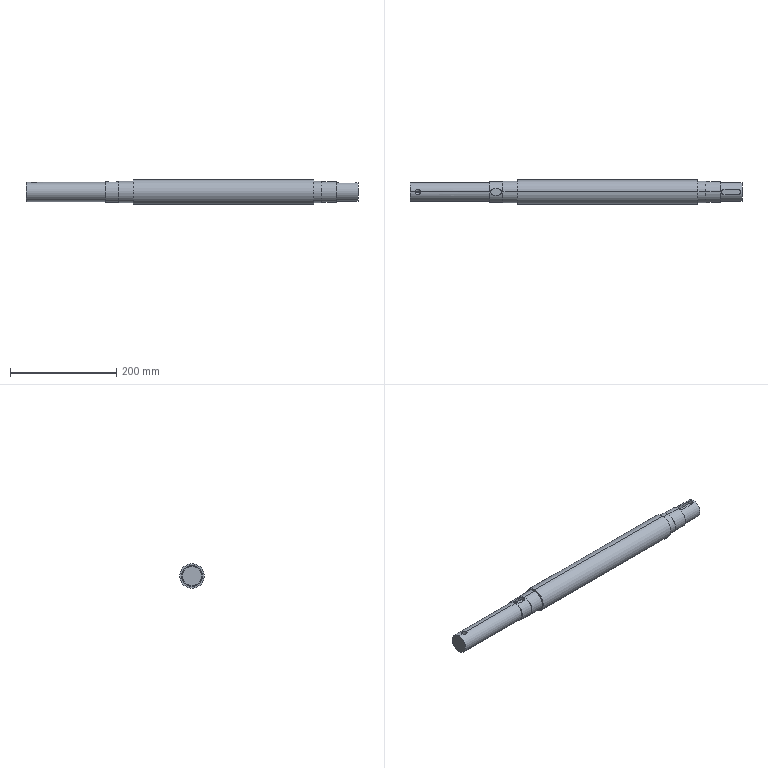Part | SolidWorks | features ICE 8, HoleWzd 2, Extrusion 1 | 1 solid | 42 faces | box 625 x 46 x 46 mm | volume 866135 mm3 | cylinder 24 | plane 14 | cone 4 | commonest cylinder face diameters 39 x4 40 x4 10 x3 12 x3 8.5 x2 10.2 x2
STEP:
#1=CARTESIAN_POINT('',(-44.,6.,18.554));
#2=VERTEX_POINT('',#1);
#3=CARTESIAN_POINT('',(-50.,0.,19.5));
#4=VERTEX_POINT('',#3);
#5=CARTESIAN_POINT('',(-44.,6.,18.554));
#6=CARTESIAN_POINT('',(-44.399,6.,18.554));
#7=CARTESIAN_POINT('',(-44.791,5.961,18.567));
#8=CARTESIAN_POINT('',(-45.369,5.845,18.603));
#9=CARTESIAN_POINT('',(-45.56,5.797,18.618));
#10=CARTESIAN_POINT('',(-45.938,5.682,18.654));
#11=CARTESIAN_POINT('',(-46.125,5.614,18.674));
#12=CARTESIAN_POINT('',(-46.669,5.388,18.742));
#13=CARTESIAN_POINT('',(-47.013,5.203,18.794));
#14=CARTESIAN_POINT('',(-47.501,4.877,18.881));
#15=CARTESIAN_POINT('',(-47.66,4.759,18.911));
#16=CARTESIAN_POINT('',(-47.963,4.51,18.972));
#17=CARTESIAN_POINT('',(-48.107,4.378,19.003));
#18=CARTESIAN_POINT('',(-48.519,3.966,19.095));
#19=CARTESIAN_POINT('',(-48.767,3.665,19.155));
#20=CARTESIAN_POINT('',(-49.206,3.009,19.269));
#21=CARTESIAN_POINT('',(-49.39,2.664,19.321));
#22=CARTESIAN_POINT('',(-49.615,2.123,19.385));
#23=CARTESIAN_POINT('',(-49.682,1.938,19.404));
#24=CARTESIAN_POINT('',(-49.797,1.561,19.438));
#25=CARTESIAN_POINT('',(-49.845,1.367,19.453));
#26=CARTESIAN_POINT('',(-49.962,0.7854,19.488));
#27=CARTESIAN_POINT('',(-50.,0.3942,19.5));
#28=CARTESIAN_POINT('',(-50.,0.,19.5));
#29=B_SPLINE_CURVE_WITH_KNOTS('',3,(#5,#6,#7,#8,#9,#10,#11,#12,#13,#14,#15,#16,#17,#18,#19,#20,#21,#22,#23,#24,#25,#26,#27,#28),.UNSPECIFIED.,.F.,.F.,(4,2,2,2,2,2,2,2,2,2,2,4),(0.,0.00118,0.00177,0.00236,0.00354,0.00413,0.00472,0.0059,0.00708,0.00767,0.008259,0.009439),.UNSPECIFIED.);
#30=EDGE_CURVE('',#2,#4,#29,.T.);
#31=ORIENTED_EDGE('',*,*,#30,.T.);
#32=CARTESIAN_POINT('',(-50.,0.,13.55));
#33=VERTEX_POINT('',#32);
#34=CARTESIAN_POINT('',(-50.,0.,22.5));
#35=DIRECTION('',(0.,0.,-1.));
#36=VECTOR('',#35,1000.);
#37=LINE('',#34,#36);
#38=EDGE_CURVE('',#4,#33,#37,.T.);
#39=ORIENTED_EDGE('',*,*,#38,.T.);
#40=CARTESIAN_POINT('',(-44.,6.,13.55));
#41=VERTEX_POINT('',#40);
#42=CARTESIAN_POINT('',(-44.,0.,13.55));
#43=DIRECTION('',(0.,0.,1.));
#44=DIRECTION('',(1.,0.,0.));
#45=AXIS2_PLACEMENT_3D('',#42,#43,#44);
#46=CIRCLE('',#45,6.);
#47=EDGE_CURVE('',#41,#33,#46,.T.);
#48=ORIENTED_EDGE('',*,*,#47,.F.);
#49=CARTESIAN_POINT('',(-44.,6.,22.5));
#50=DIRECTION('',(0.,0.,-1.));
#51=VECTOR('',#50,1000.);
#52=LINE('',#49,#51);
#53=EDGE_CURVE('',#2,#41,#52,.T.);
#54=ORIENTED_EDGE('',*,*,#53,.F.);
#55=EDGE_LOOP('',(#31,#39,#48,#54));
#56=FACE_OUTER_BOUND('',#55,.T.);
#57=CARTESIAN_POINT('',(-44.,0.,22.5));
#58=DIRECTION('',(0.,0.,-1.));
#59=DIRECTION('',(-1.,0.,0.));
#60=AXIS2_PLACEMENT_3D('',#57,#58,#59);
#61=CYLINDRICAL_SURFACE('',#60,6.);
#62=ADVANCED_FACE('',(#56),#61,.F.);
#63=CARTESIAN_POINT('',(403.,0.,4.25));
#64=VERTEX_POINT('',#63);
#65=CARTESIAN_POINT('',(403.,0.,-4.25));
#66=VERTEX_POINT('',#65);
#67=CARTESIAN_POINT('',(403.,0.,0.));
#68=DIRECTION('',(1.,0.,0.));
#69=DIRECTION('',(0.,0.,-1.));
#70=AXIS2_PLACEMENT_3D('',#67,#68,#69);
#71=CIRCLE('',#70,4.25);
#72=EDGE_CURVE('',#64,#66,#71,.T.);
#73=ORIENTED_EDGE('',*,*,#72,.F.);
#74=CARTESIAN_POINT('',(423.,0.,4.25));
#75=VERTEX_POINT('',#74);
#76=CARTESIAN_POINT('',(423.,0.,4.25));
#77=DIRECTION('',(1.,0.,0.));
#78=VECTOR('',#77,1000.);
#79=LINE('',#76,#78);
#80=EDGE_CURVE('',#64,#75,#79,.T.);
#81=ORIENTED_EDGE('',*,*,#80,.T.);
#82=CARTESIAN_POINT('',(423.,0.,-4.25));
#83=VERTEX_POINT('',#82);
#84=CARTESIAN_POINT('',(423.,0.,0.));
#85=DIRECTION('',(1.,0.,0.));
#86=DIRECTION('',(0.,0.,-1.));
#87=AXIS2_PLACEMENT_3D('',#84,#85,#86);
#88=CIRCLE('',#87,4.25);
#89=EDGE_CURVE('',#75,#83,#88,.T.);
#90=ORIENTED_EDGE('',*,*,#89,.T.);
#91=CARTESIAN_POINT('',(423.,0.,-4.25));
#92=DIRECTION('',(1.,0.,0.));
#93=VECTOR('',#92,1000.);
#94=LINE('',#91,#93);
#95=EDGE_CURVE('',#66,#83,#94,.T.);
#96=ORIENTED_EDGE('',*,*,#95,.F.);
#97=EDGE_LOOP('',(#73,#81,#90,#96));
#98=FACE_OUTER_BOUND('',#97,.T.);
#99=CARTESIAN_POINT('',(423.,0.,0.));
#100=DIRECTION('',(1.,0.,0.));
#101=DIRECTION('',(0.,0.,-1.));
#102=AXIS2_PLACEMENT_3D('',#99,#100,#101);
#103=CYLINDRICAL_SURFACE('',#102,4.25);
#104=ADVANCED_FACE('',(#98),#103,.F.);
#105=CARTESIAN_POINT('',(400.446,0.,0.));
#106=VERTEX_POINT('',#105);
#107=CARTESIAN_POINT('',(403.,0.,-4.25));
#108=DIRECTION('',(0.515,0.,-0.8572));
#109=VECTOR('',#108,1000.);
#110=LINE('',#107,#109);
#111=EDGE_CURVE('',#106,#66,#110,.T.);
#112=ORIENTED_EDGE('',*,*,#111,.F.);
#113=CARTESIAN_POINT('',(403.,0.,4.25));
#114=DIRECTION('',(0.515,0.,0.8572));
#115=VECTOR('',#114,1000.);
#116=LINE('',#113,#115);
#117=EDGE_CURVE('',#106,#64,#116,.T.);
#118=ORIENTED_EDGE('',*,*,#117,.T.);
#119=ORIENTED_EDGE('',*,*,#72,.T.);
#120=EDGE_LOOP('',(#112,#118,#119));
#121=FACE_OUTER_BOUND('',#120,.T.);
#122=CARTESIAN_POINT('',(403.,0.,0.));
#123=DIRECTION('',(1.,0.,0.));
#124=DIRECTION('',(0.,0.,-1.));
#125=AXIS2_PLACEMENT_3D('',#122,#123,#124);
#126=CONICAL_SURFACE('',#125,4.25,1.03);
#127=ADVANCED_FACE('',(#121),#126,.F.);
#128=CARTESIAN_POINT('',(-187.,0.,-5.064));
#129=VERTEX_POINT('',#128);
#130=CARTESIAN_POINT('',(-181.9,0.,-2.));
#131=VERTEX_POINT('',#130);
#132=CARTESIAN_POINT('',(-181.9,0.,-2.));
#133=DIRECTION('',(0.8572,0.,0.515));
#134=VECTOR('',#133,1000.);
#135=LINE('',#132,#134);
#136=EDGE_CURVE('',#129,#131,#135,.T.);
#137=ORIENTED_EDGE('',*,*,#136,.F.);
#138=CARTESIAN_POINT('',(-192.1,0.,-2.));
#139=VERTEX_POINT('',#138);
#140=CARTESIAN_POINT('',(-192.1,0.,-2.));
#141=DIRECTION('',(-0.8572,0.,0.515));
#142=VECTOR('',#141,1000.);
#143=LINE('',#140,#142);
#144=EDGE_CURVE('',#129,#139,#143,.T.);
#145=ORIENTED_EDGE('',*,*,#144,.T.);
#146=CARTESIAN_POINT('',(-187.,0.,-2.));
#147=DIRECTION('',(0.,0.,1.));
#148=DIRECTION('',(1.,0.,0.));
#149=AXIS2_PLACEMENT_3D('',#146,#147,#148);
#150=CIRCLE('',#149,5.1);
#151=EDGE_CURVE('',#139,#131,#150,.T.);
#152=ORIENTED_EDGE('',*,*,#151,.T.);
#153=EDGE_LOOP('',(#137,#145,#152));
#154=FACE_OUTER_BOUND('',#153,.T.);
#155=CARTESIAN_POINT('',(-187.,0.,-2.));
#156=DIRECTION('',(0.,0.,1.));
#157=DIRECTION('',(1.,0.,0.));
#158=AXIS2_PLACEMENT_3D('',#155,#156,#157);
#159=CONICAL_SURFACE('',#158,5.1,1.03);
#160=ADVANCED_FACE('',(#154),#159,.F.);
#161=ORIENTED_EDGE('',*,*,#151,.F.);
#162=CARTESIAN_POINT('',(-192.1,0.,18.));
#163=VERTEX_POINT('',#162);
#164=CARTESIAN_POINT('',(-192.1,0.,18.));
#165=DIRECTION('',(0.,0.,1.));
#166=VECTOR('',#165,1000.);
#167=LINE('',#164,#166);
#168=EDGE_CURVE('',#139,#163,#167,.T.);
#169=ORIENTED_EDGE('',*,*,#168,.T.);
#170=CARTESIAN_POINT('',(-181.9,0.,18.));
#171=VERTEX_POINT('',#170);
#172=CARTESIAN_POINT('',(-181.9,0.,18.));
#173=CARTESIAN_POINT('',(-181.9,-0.3388,18.));
#174=CARTESIAN_POINT('',(-181.933,-0.6717,17.99));
#175=CARTESIAN_POINT('',(-182.064,-1.326,17.954));
#176=CARTESIAN_POINT('',(-182.163,-1.651,17.927));
#177=CARTESIAN_POINT('',(-182.42,-2.268,17.859));
#178=CARTESIAN_POINT('',(-182.577,-2.56,17.819));
#179=CARTESIAN_POINT('',(-182.947,-3.113,17.731));
#180=CARTESIAN_POINT('',(-183.161,-3.374,17.683));
#181=CARTESIAN_POINT('',(-183.629,-3.841,17.587));
#182=CARTESIAN_POINT('',(-183.885,-4.052,17.539));
#183=CARTESIAN_POINT('',(-184.442,-4.425,17.449));
#184=CARTESIAN_POINT('',(-184.736,-4.582,17.408));
#185=CARTESIAN_POINT('',(-185.195,-4.773,17.356));
#186=CARTESIAN_POINT('',(-185.352,-4.829,17.34));
#187=CARTESIAN_POINT('',(-185.672,-4.927,17.313));
#188=CARTESIAN_POINT('',(-185.837,-4.968,17.301));
#189=CARTESIAN_POINT('',(-186.331,-5.067,17.272));
#190=CARTESIAN_POINT('',(-186.663,-5.1,17.262));
#191=CARTESIAN_POINT('',(-187.332,-5.1,17.262));
#192=CARTESIAN_POINT('',(-187.672,-5.067,17.272));
#193=CARTESIAN_POINT('',(-188.328,-4.935,17.31));
#194=CARTESIAN_POINT('',(-188.647,-4.839,17.338));
#195=CARTESIAN_POINT('',(-189.266,-4.581,17.408));
#196=CARTESIAN_POINT('',(-189.562,-4.422,17.449));
#197=CARTESIAN_POINT('',(-190.112,-4.054,17.539));
#198=CARTESIAN_POINT('',(-190.372,-3.841,17.587));
#199=CARTESIAN_POINT('',(-190.843,-3.369,17.683));
#200=CARTESIAN_POINT('',(-191.053,-3.114,17.731));
#201=CARTESIAN_POINT('',(-191.422,-2.563,17.819));
#202=CARTESIAN_POINT('',(-191.582,-2.264,17.86));
#203=CARTESIAN_POINT('',(-191.838,-1.649,17.927));
#204=CARTESIAN_POINT('',(-191.935,-1.331,17.954));
#205=CARTESIAN_POINT('',(-192.034,-0.837,17.981));
#206=CARTESIAN_POINT('',(-192.059,-0.6688,17.988));
#207=CARTESIAN_POINT('',(-192.092,-0.3341,17.998));
#208=CARTESIAN_POINT('',(-192.1,-0.167,18.));
#209=CARTESIAN_POINT('',(-192.1,0.,18.));
#210=B_SPLINE_CURVE_WITH_KNOTS('',3,(#172,#173,#174,#175,#176,#177,#178,#179,#180,#181,#182,#183,#184,#185,#186,#187,#188,#189,#190,#191,#192,#193,#194,#195,#196,#197,#198,#199,#200,#201,#202,#203,#204,#205,#206,#207,#208,#209),.UNSPECIFIED.,.F.,.F.,(4,2,2,2,2,2,2,2,2,2,2,2,2,2,2,2,2,2,4),(0.,0.001002,0.002003,0.003005,0.004007,0.005009,0.00601,0.006511,0.007012,0.008014,0.009015,0.01002,0.01102,0.01202,0.01302,0.01402,0.01503,0.01553,0.01603),.UNSPECIFIED.);
#211=EDGE_CURVE('',#171,#163,#210,.T.);
#212=ORIENTED_EDGE('',*,*,#211,.F.);
#213=CARTESIAN_POINT('',(-181.9,0.,18.));
#214=DIRECTION('',(0.,0.,1.));
#215=VECTOR('',#214,1000.);
#216=LINE('',#213,#215);
#217=EDGE_CURVE('',#131,#171,#216,.T.);
#218=ORIENTED_EDGE('',*,*,#217,.F.);
#219=EDGE_LOOP('',(#161,#169,#212,#218));
#220=FACE_OUTER_BOUND('',#219,.T.);
#221=CARTESIAN_POINT('',(-187.,0.,18.));
#222=DIRECTION('',(0.,0.,1.));
#223=DIRECTION('',(1.,0.,0.));
#224=AXIS2_PLACEMENT_3D('',#221,#222,#223);
#225=CYLINDRICAL_SURFACE('',#224,5.1);
#226=ADVANCED_FACE('',(#220),#225,.F.);
#227=CARTESIAN_POINT('',(-202.,0.,18.));
#228=VERTEX_POINT('',#227);
#229=CARTESIAN_POINT('',(-202.,0.,-18.));
#230=VERTEX_POINT('',#229);
#231=CARTESIAN_POINT('',(-202.,0.,0.));
#232=DIRECTION('',(-1.,0.,0.));
#233=DIRECTION('',(0.,0.,1.));
#234=AXIS2_PLACEMENT_3D('',#231,#232,#233);
#235=CIRCLE('',#234,18.);
#236=EDGE_CURVE('',#228,#230,#235,.T.);
#237=ORIENTED_EDGE('',*,*,#236,.F.);
#238=CARTESIAN_POINT('',(-202.,0.,18.));
#239=DIRECTION('',(1.,0.,0.));
#240=VECTOR('',#239,1000.);
#241=LINE('',#238,#240);
#242=EDGE_CURVE('',#228,#163,#241,.T.);
#243=ORIENTED_EDGE('',*,*,#242,.T.);
#244=CARTESIAN_POINT('',(-192.1,0.,18.));
#245=CARTESIAN_POINT('',(-192.1,0.3338,18.));
#246=CARTESIAN_POINT('',(-192.067,0.668,17.991));
#247=CARTESIAN_POINT('',(-191.935,1.33,17.954));
#248=CARTESIAN_POINT('',(-191.837,1.649,17.927));
#249=CARTESIAN_POINT('',(-191.582,2.264,17.86));
#250=CARTESIAN_POINT('',(-191.422,2.562,17.819));
#251=CARTESIAN_POINT('',(-191.052,3.115,17.731));
#252=CARTESIAN_POINT('',(-190.842,3.37,17.683));
#253=CARTESIAN_POINT('',(-190.489,3.723,17.611));
#254=CARTESIAN_POINT('',(-190.365,3.836,17.587));
#255=CARTESIAN_POINT('',(-190.107,4.047,17.539));
#256=CARTESIAN_POINT('',(-189.974,4.146,17.516));
#257=CARTESIAN_POINT('',(-189.562,4.422,17.449));
#258=CARTESIAN_POINT('',(-189.27,4.58,17.408));
#259=CARTESIAN_POINT('',(-188.648,4.838,17.338));
#260=CARTESIAN_POINT('',(-188.328,4.935,17.31));
#261=CARTESIAN_POINT('',(-187.838,5.033,17.282));
#262=CARTESIAN_POINT('',(-187.673,5.058,17.275));
#263=CARTESIAN_POINT('',(-187.339,5.092,17.265));
#264=CARTESIAN_POINT('',(-187.169,5.1,17.262));
#265=CARTESIAN_POINT('',(-186.665,5.1,17.262));
#266=CARTESIAN_POINT('',(-186.332,5.067,17.272));
#267=CARTESIAN_POINT('',(-185.676,4.937,17.31));
#268=CARTESIAN_POINT('',(-185.351,4.837,17.338));
#269=CARTESIAN_POINT('',(-184.736,4.582,17.408));
#270=CARTESIAN_POINT('',(-184.443,4.426,17.449));
#271=CARTESIAN_POINT('',(-183.886,4.053,17.539));
#272=CARTESIAN_POINT('',(-183.629,3.842,17.587));
#273=CARTESIAN_POINT('',(-183.278,3.491,17.659));
#274=CARTESIAN_POINT('',(-183.167,3.368,17.682));
#275=CARTESIAN_POINT('',(-182.956,3.111,17.73));
#276=CARTESIAN_POINT('',(-182.855,2.976,17.753));
#277=CARTESIAN_POINT('',(-182.577,2.561,17.819));
#278=CARTESIAN_POINT('',(-182.42,2.269,17.859));
#279=CARTESIAN_POINT('',(-182.164,1.654,17.926));
#280=CARTESIAN_POINT('',(-182.065,1.329,17.954));
#281=CARTESIAN_POINT('',(-181.933,0.6722,17.99));
#282=CARTESIAN_POINT('',(-181.9,0.3387,18.));
#283=CARTESIAN_POINT('',(-181.9,0.,18.));
#284=B_SPLINE_CURVE_WITH_KNOTS('',3,(#244,#245,#246,#247,#248,#249,#250,#251,#252,#253,#254,#255,#256,#257,#258,#259,#260,#261,#262,#263,#264,#265,#266,#267,#268,#269,#270,#271,#272,#273,#274,#275,#276,#277,#278,#279,#280,#281,#282,#283),.UNSPECIFIED.,.F.,.F.,(4,2,2,2,2,2,2,2,2,2,2,2,2,2,2,2,2,2,2,4),(0.01603,0.01703,0.01803,0.01903,0.02003,0.02053,0.02103,0.02204,0.02304,0.02354,0.02404,0.02504,0.02604,0.02704,0.02804,0.02855,0.02905,0.03005,0.03105,0.03205),.UNSPECIFIED.);
#285=EDGE_CURVE('',#163,#171,#284,.T.);
#286=ORIENTED_EDGE('',*,*,#285,.T.);
#287=CARTESIAN_POINT('',(-52.,0.,18.));
#288=VERTEX_POINT('',#287);
#289=CARTESIAN_POINT('',(-202.,0.,18.));
#290=DIRECTION('',(1.,0.,0.));
#291=VECTOR('',#290,1000.);
#292=LINE('',#289,#291);
#293=EDGE_CURVE('',#171,#288,#292,.T.);
#294=ORIENTED_EDGE('',*,*,#293,.T.);
#295=CARTESIAN_POINT('',(-52.,0.,-18.));
#296=VERTEX_POINT('',#295);
#297=CARTESIAN_POINT('',(-52.,0.,0.));
#298=DIRECTION('',(-1.,0.,0.));
#299=DIRECTION('',(0.,0.,1.));
#300=AXIS2_PLACEMENT_3D('',#297,#298,#299);
#301=CIRCLE('',#300,18.);
#302=EDGE_CURVE('',#288,#296,#301,.T.);
#303=ORIENTED_EDGE('',*,*,#302,.T.);
#304=CARTESIAN_POINT('',(-202.,0.,-18.));
#305=DIRECTION('',(1.,0.,0.));
#306=VECTOR('',#305,1000.);
#307=LINE('',#304,#306);
#308=EDGE_CURVE('',#230,#296,#307,.T.);
#309=ORIENTED_EDGE('',*,*,#308,.F.);
#310=EDGE_LOOP('',(#237,#243,#286,#294,#303,#309));
#311=FACE_OUTER_BOUND('',#310,.T.);
#312=CARTESIAN_POINT('',(-202.,0.,0.));
#313=DIRECTION('',(1.,0.,0.));
#314=DIRECTION('',(0.,0.,-1.));
#315=AXIS2_PLACEMENT_3D('',#312,#313,#314);
#316=CYLINDRICAL_SURFACE('',#315,18.);
#317=ADVANCED_FACE('',(#311),#316,.T.);
#318=CARTESIAN_POINT('',(420.,0.,11.77));
#319=VERTEX_POINT('',#318);
#320=CARTESIAN_POINT('',(415.,5.,11.77));
#321=VERTEX_POINT('',#320);
#322=CARTESIAN_POINT('',(415.,0.,11.77));
#323=DIRECTION('',(0.,0.,1.));
#324=DIRECTION('',(1.,0.,0.));
#325=AXIS2_PLACEMENT_3D('',#322,#323,#324);
#326=CIRCLE('',#325,5.);
#327=EDGE_CURVE('',#319,#321,#326,.T.);
#328=ORIENTED_EDGE('',*,*,#327,.F.);
#329=CARTESIAN_POINT('',(420.,0.,17.5));
#330=VERTEX_POINT('',#329);
#331=CARTESIAN_POINT('',(420.,0.,11.77));
#332=DIRECTION('',(0.,0.,1.));
#333=VECTOR('',#332,1000.);
#334=LINE('',#331,#333);
#335=EDGE_CURVE('',#319,#330,#334,.T.);
#336=ORIENTED_EDGE('',*,*,#335,.T.);
#337=CARTESIAN_POINT('',(415.,5.,16.771));
#338=VERTEX_POINT('',#337);
#339=CARTESIAN_POINT('',(415.,5.,16.771));
#340=CARTESIAN_POINT('',(415.332,5.,16.771));
#341=CARTESIAN_POINT('',(415.659,4.967,16.78));
#342=CARTESIAN_POINT('',(416.3,4.839,16.818));
#343=CARTESIAN_POINT('',(416.619,4.742,16.846));
#344=CARTESIAN_POINT('',(417.224,4.49,16.915));
#345=CARTESIAN_POINT('',(417.51,4.337,16.955));
#346=CARTESIAN_POINT('',(418.052,3.974,17.044));
#347=CARTESIAN_POINT('',(418.308,3.764,17.092));
#348=CARTESIAN_POINT('',(418.766,3.305,17.187));
#349=CARTESIAN_POINT('',(418.973,3.054,17.234));
#350=CARTESIAN_POINT('',(419.338,2.507,17.322));
#351=CARTESIAN_POINT('',(419.492,2.219,17.361));
#352=CARTESIAN_POINT('',(419.68,1.768,17.411));
#353=CARTESIAN_POINT('',(419.735,1.614,17.426));
#354=CARTESIAN_POINT('',(419.831,1.3,17.452));
#355=CARTESIAN_POINT('',(419.871,1.139,17.464));
#356=CARTESIAN_POINT('',(419.968,0.6539,17.491));
#357=CARTESIAN_POINT('',(420.,0.3282,17.5));
#358=CARTESIAN_POINT('',(420.,0.,17.5));
#359=B_SPLINE_CURVE_WITH_KNOTS('',3,(#339,#340,#341,#342,#343,#344,#345,#346,#347,#348,#349,#350,#351,#352,#353,#354,#355,#356,#357,#358),.UNSPECIFIED.,.F.,.F.,(4,2,2,2,2,2,2,2,2,4),(0.,0.0009824,0.001965,0.002947,0.00393,0.004912,0.005894,0.006386,0.006877,0.007859),.UNSPECIFIED.);
#360=EDGE_CURVE('',#338,#330,#359,.T.);
#361=ORIENTED_EDGE('',*,*,#360,.F.);
#362=CARTESIAN_POINT('',(415.,5.,11.77));
#363=DIRECTION('',(0.,0.,1.));
#364=VECTOR('',#363,1000.);
#365=LINE('',#362,#364);
#366=EDGE_CURVE('',#321,#338,#365,.T.);
#367=ORIENTED_EDGE('',*,*,#366,.F.);
#368=EDGE_LOOP('',(#328,#336,#361,#367));
#369=FACE_OUTER_BOUND('',#368,.T.);
#370=CARTESIAN_POINT('',(415.,0.,11.77));
#371=DIRECTION('',(0.,0.,1.));
#372=DIRECTION('',(1.,0.,0.));
#373=AXIS2_PLACEMENT_3D('',#370,#371,#372);
#374=CYLINDRICAL_SURFACE('',#373,5.);
#375=ADVANCED_FACE('',(#369),#374,.F.);
#376=CARTESIAN_POINT('',(423.,0.,-17.5));
#377=VERTEX_POINT('',#376);
#378=CARTESIAN_POINT('',(423.,0.,17.5));
#379=VERTEX_POINT('',#378);
#380=CARTESIAN_POINT('',(423.,0.,0.));
#381=DIRECTION('',(1.,0.,0.));
#382=DIRECTION('',(0.,0.,-1.));
#383=AXIS2_PLACEMENT_3D('',#380,#381,#382);
#384=CIRCLE('',#383,17.5);
#385=EDGE_CURVE('',#377,#379,#384,.T.);
#386=ORIENTED_EDGE('',*,*,#385,.F.);
#387=CARTESIAN_POINT('',(382.,0.,-17.5));
#388=VERTEX_POINT('',#387);
#389=CARTESIAN_POINT('',(423.,0.,-17.5));
#390=DIRECTION('',(-1.,0.,0.));
#391=VECTOR('',#390,1000.);
#392=LINE('',#389,#391);
#393=EDGE_CURVE('',#377,#388,#392,.T.);
#394=ORIENTED_EDGE('',*,*,#393,.T.);
#395=CARTESIAN_POINT('',(382.,0.,17.5));
#396=VERTEX_POINT('',#395);
#397=CARTESIAN_POINT('',(382.,0.,0.));
#398=DIRECTION('',(1.,0.,0.));
#399=DIRECTION('',(0.,0.,-1.));
#400=AXIS2_PLACEMENT_3D('',#397,#398,#399);
#401=CIRCLE('',#400,17.5);
#402=EDGE_CURVE('',#388,#396,#401,.T.);
#403=ORIENTED_EDGE('',*,*,#402,.T.);
#404=CARTESIAN_POINT('',(384.,0.,17.5));
#405=VERTEX_POINT('',#404);
#406=CARTESIAN_POINT('',(423.,0.,17.5));
#407=DIRECTION('',(-1.,0.,0.));
#408=VECTOR('',#407,1000.);
#409=LINE('',#406,#408);
#410=EDGE_CURVE('',#405,#396,#409,.T.);
#411=ORIENTED_EDGE('',*,*,#410,.F.);
#412=CARTESIAN_POINT('',(389.,5.,16.771));
#413=VERTEX_POINT('',#412);
#414=CARTESIAN_POINT('',(384.,0.,17.5));
#415=CARTESIAN_POINT('',(384.,0.3278,17.5));
#416=CARTESIAN_POINT('',(384.033,0.6608,17.49));
#417=CARTESIAN_POINT('',(384.162,1.303,17.454));
#418=CARTESIAN_POINT('',(384.257,1.615,17.428));
#419=CARTESIAN_POINT('',(384.509,2.222,17.361));
#420=CARTESIAN_POINT('',(384.665,2.512,17.321));
#421=CARTESIAN_POINT('',(385.026,3.051,17.234));
#422=CARTESIAN_POINT('',(385.234,3.305,17.187));
#423=CARTESIAN_POINT('',(385.696,3.767,17.091));
#424=CARTESIAN_POINT('',(385.946,3.972,17.044));
#425=CARTESIAN_POINT('',(386.486,4.334,16.956));
#426=CARTESIAN_POINT('',(386.778,4.491,16.914));
#427=CARTESIAN_POINT('',(387.38,4.742,16.846));
#428=CARTESIAN_POINT('',(387.692,4.837,16.818));
#429=CARTESIAN_POINT('',(388.336,4.967,16.781));
#430=CARTESIAN_POINT('',(388.668,5.,16.771));
#431=CARTESIAN_POINT('',(389.,5.,16.771));
#432=B_SPLINE_CURVE_WITH_KNOTS('',3,(#414,#415,#416,#417,#418,#419,#420,#421,#422,#423,#424,#425,#426,#427,#428,#429,#430,#431),.UNSPECIFIED.,.F.,.F.,(4,2,2,2,2,2,2,2,4),(0.007859,0.008841,0.009822,0.0108,0.01178,0.01277,0.01375,0.01473,0.01571),.UNSPECIFIED.);
#433=EDGE_CURVE('',#405,#413,#432,.T.);
#434=ORIENTED_EDGE('',*,*,#433,.T.);
#435=CARTESIAN_POINT('',(423.,5.,16.771));
#436=DIRECTION('',(1.,0.,0.));
#437=VECTOR('',#436,1000.);
#438=LINE('',#435,#437);
#439=EDGE_CURVE('',#413,#338,#438,.T.);
#440=ORIENTED_EDGE('',*,*,#439,.T.);
#441=ORIENTED_EDGE('',*,*,#360,.T.);
#442=CARTESIAN_POINT('',(423.,0.,17.5));
#443=DIRECTION('',(-1.,0.,0.));
#444=VECTOR('',#443,1000.);
#445=LINE('',#442,#444);
#446=EDGE_CURVE('',#379,#330,#445,.T.);
#447=ORIENTED_EDGE('',*,*,#446,.F.);
#448=EDGE_LOOP('',(#386,#394,#403,#411,#434,#440,#441,#447));
#449=FACE_OUTER_BOUND('',#448,.T.);
#450=CARTESIAN_POINT('',(423.,0.,0.));
#451=DIRECTION('',(-1.,0.,0.));
#452=DIRECTION('',(0.,0.,1.));
#453=AXIS2_PLACEMENT_3D('',#450,#451,#452);
#454=CYLINDRICAL_SURFACE('',#453,17.5);
#455=ADVANCED_FACE('',(#449),#454,.T.);
#456=CARTESIAN_POINT('',(382.,0.,-19.5));
#457=VERTEX_POINT('',#456);
#458=CARTESIAN_POINT('',(382.,0.,19.5));
#459=VERTEX_POINT('',#458);
#460=CARTESIAN_POINT('',(382.,0.,0.));
#461=DIRECTION('',(1.,0.,0.));
#462=DIRECTION('',(0.,0.,-1.));
#463=AXIS2_PLACEMENT_3D('',#460,#461,#462);
#464=CIRCLE('',#463,19.5);
#465=EDGE_CURVE('',#457,#459,#464,.T.);
#466=ORIENTED_EDGE('',*,*,#465,.F.);
#467=CARTESIAN_POINT('',(355.,0.,-19.5));
#468=VERTEX_POINT('',#467);
#469=CARTESIAN_POINT('',(382.,0.,-19.5));
#470=DIRECTION('',(-1.,0.,0.));
#471=VECTOR('',#470,1000.);
#472=LINE('',#469,#471);
#473=EDGE_CURVE('',#457,#468,#472,.T.);
#474=ORIENTED_EDGE('',*,*,#473,.T.);
#475=CARTESIAN_POINT('',(355.,0.,19.5));
#476=VERTEX_POINT('',#475);
#477=CARTESIAN_POINT('',(355.,0.,0.));
#478=DIRECTION('',(1.,0.,0.));
#479=DIRECTION('',(0.,0.,-1.));
#480=AXIS2_PLACEMENT_3D('',#477,#478,#479);
#481=CIRCLE('',#480,19.5);
#482=EDGE_CURVE('',#468,#476,#481,.T.);
#483=ORIENTED_EDGE('',*,*,#482,.T.);
#484=CARTESIAN_POINT('',(382.,0.,19.5));
#485=DIRECTION('',(-1.,0.,0.));
#486=VECTOR('',#485,1000.);
#487=LINE('',#484,#486);
#488=EDGE_CURVE('',#459,#476,#487,.T.);
#489=ORIENTED_EDGE('',*,*,#488,.F.);
#490=EDGE_LOOP('',(#466,#474,#483,#489));
#491=FACE_OUTER_BOUND('',#490,.T.);
#492=CARTESIAN_POINT('',(382.,0.,0.));
#493=DIRECTION('',(-1.,0.,0.));
#494=DIRECTION('',(0.,0.,1.));
#495=AXIS2_PLACEMENT_3D('',#492,#493,#494);
#496=CYLINDRICAL_SURFACE('',#495,19.5);
#497=ADVANCED_FACE('',(#491),#496,.T.);
#498=CARTESIAN_POINT('',(355.,0.,-20.));
#499=VERTEX_POINT('',#498);
#500=CARTESIAN_POINT('',(355.,0.,20.));
#501=VERTEX_POINT('',#500);
#502=CARTESIAN_POINT('',(355.,0.,0.));
#503=DIRECTION('',(1.,0.,0.));
#504=DIRECTION('',(0.,0.,-1.));
#505=AXIS2_PLACEMENT_3D('',#502,#503,#504);
#506=CIRCLE('',#505,20.);
#507=EDGE_CURVE('',#499,#501,#506,.T.);
#508=ORIENTED_EDGE('',*,*,#507,.F.);
#509=CARTESIAN_POINT('',(340.,0.,-20.));
#510=VERTEX_POINT('',#509);
#511=CARTESIAN_POINT('',(355.,0.,-20.));
#512=DIRECTION('',(-1.,0.,0.));
#513=VECTOR('',#512,1000.);
#514=LINE('',#511,#513);
#515=EDGE_CURVE('',#499,#510,#514,.T.);
#516=ORIENTED_EDGE('',*,*,#515,.T.);
#517=CARTESIAN_POINT('',(340.,0.,20.));
#518=VERTEX_POINT('',#517);
#519=CARTESIAN_POINT('',(340.,0.,0.));
#520=DIRECTION('',(1.,0.,0.));
#521=DIRECTION('',(0.,0.,-1.));
#522=AXIS2_PLACEMENT_3D('',#519,#520,#521);
#523=CIRCLE('',#522,20.);
#524=EDGE_CURVE('',#510,#518,#523,.T.);
#525=ORIENTED_EDGE('',*,*,#524,.T.);
#526=CARTESIAN_POINT('',(355.,0.,20.));
#527=DIRECTION('',(-1.,0.,0.));
#528=VECTOR('',#527,1000.);
#529=LINE('',#526,#528);
#530=EDGE_CURVE('',#501,#518,#529,.T.);
#531=ORIENTED_EDGE('',*,*,#530,.F.);
#532=EDGE_LOOP('',(#508,#516,#525,#531));
#533=FACE_OUTER_BOUND('',#532,.T.);
#534=CARTESIAN_POINT('',(355.,0.,0.));
#535=DIRECTION('',(-1.,0.,0.));
#536=DIRECTION('',(0.,0.,1.));
#537=AXIS2_PLACEMENT_3D('',#534,#535,#536);
#538=CYLINDRICAL_SURFACE('',#537,20.);
#539=ADVANCED_FACE('',(#533),#538,.T.);
#540=CARTESIAN_POINT('',(-27.,0.,20.));
#541=VERTEX_POINT('',#540);
#542=CARTESIAN_POINT('',(-27.,0.,-20.));
#543=VERTEX_POINT('',#542);
#544=CARTESIAN_POINT('',(-27.,0.,0.));
#545=DIRECTION('',(-1.,0.,0.));
#546=DIRECTION('',(0.,0.,1.));
#547=AXIS2_PLACEMENT_3D('',#544,#545,#546);
#548=CIRCLE('',#547,20.);
#549=EDGE_CURVE('',#541,#543,#548,.T.);
#550=ORIENTED_EDGE('',*,*,#549,.F.);
#551=CARTESIAN_POINT('',(0.,0.,20.));
#552=VERTEX_POINT('',#551);
#553=CARTESIAN_POINT('',(-27.,0.,20.));
#554=DIRECTION('',(1.,0.,0.));
#555=VECTOR('',#554,1000.);
#556=LINE('',#553,#555);
#557=EDGE_CURVE('',#541,#552,#556,.T.);
#558=ORIENTED_EDGE('',*,*,#557,.T.);
#559=CARTESIAN_POINT('',(0.,0.,-20.));
#560=VERTEX_POINT('',#559);
#561=CARTESIAN_POINT('',(0.,0.,0.));
#562=DIRECTION('',(-1.,0.,0.));
#563=DIRECTION('',(0.,0.,-1.));
#564=AXIS2_PLACEMENT_3D('',#561,#562,#563);
#565=CIRCLE('',#564,20.);
#566=EDGE_CURVE('',#552,#560,#565,.T.);
#567=ORIENTED_EDGE('',*,*,#566,.T.);
#568=CARTESIAN_POINT('',(-27.,0.,-20.));
#569=DIRECTION('',(1.,0.,0.));
#570=VECTOR('',#569,1000.);
#571=LINE('',#568,#570);
#572=EDGE_CURVE('',#543,#560,#571,.T.);
#573=ORIENTED_EDGE('',*,*,#572,.F.);
#574=EDGE_LOOP('',(#550,#558,#567,#573));
#575=FACE_OUTER_BOUND('',#574,.T.);
#576=CARTESIAN_POINT('',(-27.,0.,0.));
#577=DIRECTION('',(1.,0.,0.));
#578=DIRECTION('',(0.,0.,-1.));
#579=AXIS2_PLACEMENT_3D('',#576,#577,#578);
#580=CYLINDRICAL_SURFACE('',#579,20.);
#581=ADVANCED_FACE('',(#575),#580,.T.);
#582=CARTESIAN_POINT('',(340.,0.,-23.));
#583=VERTEX_POINT('',#582);
#584=CARTESIAN_POINT('',(340.,0.,23.));
#585=VERTEX_POINT('',#584);
#586=CARTESIAN_POINT('',(340.,0.,0.));
#587=DIRECTION('',(1.,0.,0.));
#588=DIRECTION('',(0.,0.,-1.));
#589=AXIS2_PLACEMENT_3D('',#586,#587,#588);
#590=CIRCLE('',#589,23.);
#591=EDGE_CURVE('',#583,#585,#590,.T.);
#592=ORIENTED_EDGE('',*,*,#591,.F.);
#593=CARTESIAN_POINT('',(0.,0.,-23.));
#594=VERTEX_POINT('',#593);
#595=CARTESIAN_POINT('',(340.,0.,-23.));
#596=DIRECTION('',(-1.,0.,0.));
#597=VECTOR('',#596,1000.);
#598=LINE('',#595,#597);
#599=EDGE_CURVE('',#583,#594,#598,.T.);
#600=ORIENTED_EDGE('',*,*,#599,.T.);
#601=CARTESIAN_POINT('',(0.,0.,23.));
#602=VERTEX_POINT('',#601);
#603=CARTESIAN_POINT('',(0.,0.,0.));
#604=DIRECTION('',(1.,0.,0.));
#605=DIRECTION('',(0.,0.,-1.));
#606=AXIS2_PLACEMENT_3D('',#603,#604,#605);
#607=CIRCLE('',#606,23.);
#608=EDGE_CURVE('',#594,#602,#607,.T.);
#609=ORIENTED_EDGE('',*,*,#608,.T.);
#610=CARTESIAN_POINT('',(340.,0.,23.));
#611=DIRECTION('',(-1.,0.,0.));
#612=VECTOR('',#611,1000.);
#613=LINE('',#610,#612);
#614=EDGE_CURVE('',#585,#602,#613,.T.);
#615=ORIENTED_EDGE('',*,*,#614,.F.);
#616=EDGE_LOOP('',(#592,#600,#609,#615));
#617=FACE_OUTER_BOUND('',#616,.T.);
#618=CARTESIAN_POINT('',(340.,0.,0.));
#619=DIRECTION('',(-1.,0.,0.));
#620=DIRECTION('',(0.,0.,1.));
#621=AXIS2_PLACEMENT_3D('',#618,#619,#620);
#622=CYLINDRICAL_SURFACE('',#621,23.);
#623=ADVANCED_FACE('',(#617),#622,.T.);
#624=CARTESIAN_POINT('',(-52.,0.,19.5));
#625=VERTEX_POINT('',#624);
#626=CARTESIAN_POINT('',(-52.,0.,-19.5));
#627=VERTEX_POINT('',#626);
#628=CARTESIAN_POINT('',(-52.,0.,0.));
#629=DIRECTION('',(-1.,0.,0.));
#630=DIRECTION('',(0.,0.,1.));
#631=AXIS2_PLACEMENT_3D('',#628,#629,#630);
#632=CIRCLE('',#631,19.5);
#633=EDGE_CURVE('',#625,#627,#632,.T.);
#634=ORIENTED_EDGE('',*,*,#633,.F.);
#635=CARTESIAN_POINT('',(-52.,0.,19.5));
#636=DIRECTION('',(1.,0.,0.));
#637=VECTOR('',#636,1000.);
#638=LINE('',#635,#637);
#639=EDGE_CURVE('',#625,#4,#638,.T.);
#640=ORIENTED_EDGE('',*,*,#639,.T.);
#641=ORIENTED_EDGE('',*,*,#30,.F.);
#642=CARTESIAN_POINT('',(-36.,6.,18.554));
#643=VERTEX_POINT('',#642);
#644=CARTESIAN_POINT('',(-52.,6.,18.554));
#645=DIRECTION('',(-1.,0.,0.));
#646=VECTOR('',#645,1000.);
#647=LINE('',#644,#646);
#648=EDGE_CURVE('',#643,#2,#647,.T.);
#649=ORIENTED_EDGE('',*,*,#648,.F.);
#650=CARTESIAN_POINT('',(-30.,0.,19.5));
#651=VERTEX_POINT('',#650);
#652=CARTESIAN_POINT('',(-30.,0.,19.5));
#653=CARTESIAN_POINT('',(-30.,0.3937,19.5));
#654=CARTESIAN_POINT('',(-30.04,0.7937,19.488));
#655=CARTESIAN_POINT('',(-30.194,1.565,19.441));
#656=CARTESIAN_POINT('',(-30.308,1.939,19.407));
#657=CARTESIAN_POINT('',(-30.612,2.668,19.32));
#658=CARTESIAN_POINT('',(-30.798,3.015,19.268));
#659=CARTESIAN_POINT('',(-31.123,3.5,19.184));
#660=CARTESIAN_POINT('',(-31.239,3.657,19.155));
#661=CARTESIAN_POINT('',(-31.487,3.959,19.095));
#662=CARTESIAN_POINT('',(-31.62,4.105,19.063));
#663=CARTESIAN_POINT('',(-32.035,4.52,18.971));
#664=CARTESIAN_POINT('',(-32.335,4.766,18.91));
#665=CARTESIAN_POINT('',(-32.982,5.2,18.795));
#666=CARTESIAN_POINT('',(-33.333,5.389,18.741));
#667=CARTESIAN_POINT('',(-34.055,5.689,18.652));
#668=CARTESIAN_POINT('',(-34.429,5.804,18.616));
#669=CARTESIAN_POINT('',(-35.203,5.96,18.567));
#670=CARTESIAN_POINT('',(-35.601,6.,18.554));
#671=CARTESIAN_POINT('',(-36.,6.,18.554));
#672=B_SPLINE_CURVE_WITH_KNOTS('',3,(#652,#653,#654,#655,#656,#657,#658,#659,#660,#661,#662,#663,#664,#665,#666,#667,#668,#669,#670,#671),.UNSPECIFIED.,.F.,.F.,(4,2,2,2,2,2,2,2,2,4),(0.009439,0.01062,0.0118,0.01297,0.01356,0.01415,0.01533,0.01651,0.01769,0.01887),.UNSPECIFIED.);
#673=EDGE_CURVE('',#651,#643,#672,.T.);
#674=ORIENTED_EDGE('',*,*,#673,.F.);
#675=CARTESIAN_POINT('',(-27.,0.,19.5));
#676=VERTEX_POINT('',#675);
#677=CARTESIAN_POINT('',(-52.,0.,19.5));
#678=DIRECTION('',(1.,0.,0.));
#679=VECTOR('',#678,1000.);
#680=LINE('',#677,#679);
#681=EDGE_CURVE('',#651,#676,#680,.T.);
#682=ORIENTED_EDGE('',*,*,#681,.T.);
#683=CARTESIAN_POINT('',(-27.,0.,-19.5));
#684=VERTEX_POINT('',#683);
#685=CARTESIAN_POINT('',(-27.,0.,0.));
#686=DIRECTION('',(-1.,0.,0.));
#687=DIRECTION('',(0.,0.,1.));
#688=AXIS2_PLACEMENT_3D('',#685,#686,#687);
#689=CIRCLE('',#688,19.5);
#690=EDGE_CURVE('',#676,#684,#689,.T.);
#691=ORIENTED_EDGE('',*,*,#690,.T.);
#692=CARTESIAN_POINT('',(-52.,0.,-19.5));
#693=DIRECTION('',(1.,0.,0.));
#694=VECTOR('',#693,1000.);
#695=LINE('',#692,#694);
#696=EDGE_CURVE('',#627,#684,#695,.T.);
#697=ORIENTED_EDGE('',*,*,#696,.F.);
#698=EDGE_LOOP('',(#634,#640,#641,#649,#674,#682,#691,#697));
#699=FACE_OUTER_BOUND('',#698,.T.);
#700=CARTESIAN_POINT('',(-52.,0.,0.));
#701=DIRECTION('',(1.,0.,0.));
#702=DIRECTION('',(0.,0.,-1.));
#703=AXIS2_PLACEMENT_3D('',#700,#701,#702);
#704=CYLINDRICAL_SURFACE('',#703,19.5);
#705=ADVANCED_FACE('',(#699),#704,.T.);
#706=ORIENTED_EDGE('',*,*,#639,.F.);
#707=CARTESIAN_POINT('',(-52.,0.,0.));
#708=DIRECTION('',(-1.,0.,0.));
#709=DIRECTION('',(0.,0.,1.));
#710=AXIS2_PLACEMENT_3D('',#707,#708,#709);
#711=CIRCLE('',#710,19.5);
#712=EDGE_CURVE('',#627,#625,#711,.T.);
#713=ORIENTED_EDGE('',*,*,#712,.F.);
#714=ORIENTED_EDGE('',*,*,#696,.T.);
#715=CARTESIAN_POINT('',(-27.,0.,0.));
#716=DIRECTION('',(-1.,0.,0.));
#717=DIRECTION('',(0.,0.,1.));
#718=AXIS2_PLACEMENT_3D('',#715,#716,#717);
#719=CIRCLE('',#718,19.5);
#720=EDGE_CURVE('',#684,#676,#719,.T.);
#721=ORIENTED_EDGE('',*,*,#720,.T.);
#722=ORIENTED_EDGE('',*,*,#681,.F.);
#723=CARTESIAN_POINT('',(-36.,-6.,18.554));
#724=VERTEX_POINT('',#723);
#725=CARTESIAN_POINT('',(-36.,-6.,18.554));
#726=CARTESIAN_POINT('',(-35.601,-6.,18.554));
#727=CARTESIAN_POINT('',(-35.209,-5.961,18.567));
#728=CARTESIAN_POINT('',(-34.631,-5.845,18.603));
#729=CARTESIAN_POINT('',(-34.44,-5.797,18.618));
#730=CARTESIAN_POINT('',(-34.062,-5.682,18.654));
#731=CARTESIAN_POINT('',(-33.875,-5.614,18.674));
#732=CARTESIAN_POINT('',(-33.331,-5.388,18.742));
#733=CARTESIAN_POINT('',(-32.987,-5.203,18.794));
#734=CARTESIAN_POINT('',(-32.499,-4.877,18.881));
#735=CARTESIAN_POINT('',(-32.34,-4.759,18.911));
#736=CARTESIAN_POINT('',(-32.037,-4.51,18.972));
#737=CARTESIAN_POINT('',(-31.893,-4.378,19.003));
#738=CARTESIAN_POINT('',(-31.481,-3.966,19.095));
#739=CARTESIAN_POINT('',(-31.233,-3.665,19.155));
#740=CARTESIAN_POINT('',(-30.794,-3.009,19.269));
#741=CARTESIAN_POINT('',(-30.61,-2.664,19.321));
#742=CARTESIAN_POINT('',(-30.385,-2.123,19.385));
#743=CARTESIAN_POINT('',(-30.318,-1.938,19.404));
#744=CARTESIAN_POINT('',(-30.203,-1.561,19.438));
#745=CARTESIAN_POINT('',(-30.155,-1.367,19.453));
#746=CARTESIAN_POINT('',(-30.038,-0.7854,19.488));
#747=CARTESIAN_POINT('',(-30.,-0.3942,19.5));
#748=CARTESIAN_POINT('',(-30.,0.,19.5));
#749=B_SPLINE_CURVE_WITH_KNOTS('',3,(#725,#726,#727,#728,#729,#730,#731,#732,#733,#734,#735,#736,#737,#738,#739,#740,#741,#742,#743,#744,#745,#746,#747,#748),.UNSPECIFIED.,.F.,.F.,(4,2,2,2,2,2,2,2,2,2,2,4),(0.,0.00118,0.00177,0.00236,0.00354,0.00413,0.00472,0.0059,0.00708,0.00767,0.008259,0.009439),.UNSPECIFIED.);
#750=EDGE_CURVE('',#724,#651,#749,.T.);
#751=ORIENTED_EDGE('',*,*,#750,.F.);
#752=CARTESIAN_POINT('',(-44.,-6.,18.554));
#753=VERTEX_POINT('',#752);
#754=CARTESIAN_POINT('',(-52.,-6.,18.554));
#755=DIRECTION('',(1.,0.,0.));
#756=VECTOR('',#755,1000.);
#757=LINE('',#754,#756);
#758=EDGE_CURVE('',#753,#724,#757,.T.);
#759=ORIENTED_EDGE('',*,*,#758,.F.);
#760=CARTESIAN_POINT('',(-50.,0.,19.5));
#761=CARTESIAN_POINT('',(-50.,-0.3937,19.5));
#762=CARTESIAN_POINT('',(-49.96,-0.7937,19.488));
#763=CARTESIAN_POINT('',(-49.806,-1.565,19.441));
#764=CARTESIAN_POINT('',(-49.692,-1.939,19.407));
#765=CARTESIAN_POINT('',(-49.388,-2.668,19.32));
#766=CARTESIAN_POINT('',(-49.202,-3.015,19.268));
#767=CARTESIAN_POINT('',(-48.877,-3.5,19.184));
#768=CARTESIAN_POINT('',(-48.761,-3.657,19.155));
#769=CARTESIAN_POINT('',(-48.513,-3.959,19.095));
#770=CARTESIAN_POINT('',(-48.38,-4.105,19.063));
#771=CARTESIAN_POINT('',(-47.965,-4.52,18.971));
#772=CARTESIAN_POINT('',(-47.665,-4.766,18.91));
#773=CARTESIAN_POINT('',(-47.018,-5.2,18.795));
#774=CARTESIAN_POINT('',(-46.667,-5.389,18.741));
#775=CARTESIAN_POINT('',(-45.945,-5.689,18.652));
#776=CARTESIAN_POINT('',(-45.571,-5.804,18.616));
#777=CARTESIAN_POINT('',(-44.797,-5.96,18.567));
#778=CARTESIAN_POINT('',(-44.399,-6.,18.554));
#779=CARTESIAN_POINT('',(-44.,-6.,18.554));
#780=B_SPLINE_CURVE_WITH_KNOTS('',3,(#760,#761,#762,#763,#764,#765,#766,#767,#768,#769,#770,#771,#772,#773,#774,#775,#776,#777,#778,#779),.UNSPECIFIED.,.F.,.F.,(4,2,2,2,2,2,2,2,2,4),(0.009439,0.01062,0.0118,0.01297,0.01356,0.01415,0.01533,0.01651,0.01769,0.01887),.UNSPECIFIED.);
#781=EDGE_CURVE('',#4,#753,#780,.T.);
#782=ORIENTED_EDGE('',*,*,#781,.F.);
#783=EDGE_LOOP('',(#706,#713,#714,#721,#722,#751,#759,#782));
#784=FACE_OUTER_BOUND('',#783,.T.);
#785=CARTESIAN_POINT('',(-52.,0.,0.));
#786=DIRECTION('',(1.,0.,0.));
#787=DIRECTION('',(0.,0.,-1.));
#788=AXIS2_PLACEMENT_3D('',#785,#786,#787);
#789=CYLINDRICAL_SURFACE('',#788,19.5);
#790=ADVANCED_FACE('',(#784),#789,.T.);
#791=ORIENTED_EDGE('',*,*,#712,.T.);
#792=ORIENTED_EDGE('',*,*,#633,.T.);
#793=EDGE_LOOP('',(#791,#792));
#794=FACE_OUTER_BOUND('',#793,.T.);
#795=CARTESIAN_POINT('',(-52.,0.,0.));
#796=DIRECTION('',(-1.,0.,0.));
#797=DIRECTION('',(0.,0.,1.));
#798=AXIS2_PLACEMENT_3D('',#795,#796,#797);
#799=CIRCLE('',#798,18.);
#800=EDGE_CURVE('',#296,#288,#799,.T.);
#801=ORIENTED_EDGE('',*,*,#800,.F.);
#802=ORIENTED_EDGE('',*,*,#302,.F.);
#803=EDGE_LOOP('',(#801,#802));
#804=FACE_BOUND('',#803,.T.);
#805=CARTESIAN_POINT('',(-52.,0.,0.));
#806=DIRECTION('',(-1.,0.,0.));
#807=DIRECTION('',(0.,0.,1.));
#808=AXIS2_PLACEMENT_3D('',#805,#806,#807);
#809=PLANE('',#808);
#810=ADVANCED_FACE('',(#794,#804),#809,.T.);
#811=CARTESIAN_POINT('',(382.,0.,0.));
#812=DIRECTION('',(1.,0.,0.));
#813=DIRECTION('',(0.,0.,-1.));
#814=AXIS2_PLACEMENT_3D('',#811,#812,#813);
#815=CIRCLE('',#814,19.5);
#816=EDGE_CURVE('',#459,#457,#815,.T.);
#817=ORIENTED_EDGE('',*,*,#816,.T.);
#818=ORIENTED_EDGE('',*,*,#465,.T.);
#819=EDGE_LOOP('',(#817,#818));
#820=FACE_OUTER_BOUND('',#819,.T.);
#821=CARTESIAN_POINT('',(382.,0.,0.));
#822=DIRECTION('',(1.,0.,0.));
#823=DIRECTION('',(0.,0.,-1.));
#824=AXIS2_PLACEMENT_3D('',#821,#822,#823);
#825=CIRCLE('',#824,17.5);
#826=EDGE_CURVE('',#396,#388,#825,.T.);
#827=ORIENTED_EDGE('',*,*,#826,.F.);
#828=ORIENTED_EDGE('',*,*,#402,.F.);
#829=EDGE_LOOP('',(#827,#828));
#830=FACE_BOUND('',#829,.T.);
#831=CARTESIAN_POINT('',(382.,0.,0.));
#832=DIRECTION('',(1.,0.,0.));
#833=DIRECTION('',(0.,0.,-1.));
#834=AXIS2_PLACEMENT_3D('',#831,#832,#833);
#835=PLANE('',#834);
#836=ADVANCED_FACE('',(#820,#830),#835,.T.);
#837=CARTESIAN_POINT('',(355.,0.,0.));
#838=DIRECTION('',(1.,0.,0.));
#839=DIRECTION('',(0.,0.,-1.));
#840=AXIS2_PLACEMENT_3D('',#837,#838,#839);
#841=CIRCLE('',#840,20.);
#842=EDGE_CURVE('',#501,#499,#841,.T.);
#843=ORIENTED_EDGE('',*,*,#842,.T.);
#844=ORIENTED_EDGE('',*,*,#507,.T.);
#845=EDGE_LOOP('',(#843,#844));
#846=FACE_OUTER_BOUND('',#845,.T.);
#847=CARTESIAN_POINT('',(355.,0.,0.));
#848=DIRECTION('',(1.,0.,0.));
#849=DIRECTION('',(0.,0.,-1.));
#850=AXIS2_PLACEMENT_3D('',#847,#848,#849);
#851=CIRCLE('',#850,19.5);
#852=EDGE_CURVE('',#476,#468,#851,.T.);
#853=ORIENTED_EDGE('',*,*,#852,.F.);
#854=ORIENTED_EDGE('',*,*,#482,.F.);
#855=EDGE_LOOP('',(#853,#854));
#856=FACE_BOUND('',#855,.T.);
#857=CARTESIAN_POINT('',(355.,0.,0.));
#858=DIRECTION('',(1.,0.,0.));
#859=DIRECTION('',(0.,0.,-1.));
#860=AXIS2_PLACEMENT_3D('',#857,#858,#859);
#861=PLANE('',#860);
#862=ADVANCED_FACE('',(#846,#856),#861,.T.);
#863=CARTESIAN_POINT('',(340.,0.,0.));
#864=DIRECTION('',(1.,0.,0.));
#865=DIRECTION('',(0.,0.,-1.));
#866=AXIS2_PLACEMENT_3D('',#863,#864,#865);
#867=CIRCLE('',#866,23.);
#868=EDGE_CURVE('',#585,#583,#867,.T.);
#869=ORIENTED_EDGE('',*,*,#868,.T.);
#870=ORIENTED_EDGE('',*,*,#591,.T.);
#871=EDGE_LOOP('',(#869,#870));
#872=FACE_OUTER_BOUND('',#871,.T.);
#873=CARTESIAN_POINT('',(340.,0.,0.));
#874=DIRECTION('',(1.,0.,0.));
#875=DIRECTION('',(0.,0.,-1.));
#876=AXIS2_PLACEMENT_3D('',#873,#874,#875);
#877=CIRCLE('',#876,20.);
#878=EDGE_CURVE('',#518,#510,#877,.T.);
#879=ORIENTED_EDGE('',*,*,#878,.F.);
#880=ORIENTED_EDGE('',*,*,#524,.F.);
#881=EDGE_LOOP('',(#879,#880));
#882=FACE_BOUND('',#881,.T.);
#883=CARTESIAN_POINT('',(340.,0.,0.));
#884=DIRECTION('',(1.,0.,0.));
#885=DIRECTION('',(0.,0.,-1.));
#886=AXIS2_PLACEMENT_3D('',#883,#884,#885);
#887=PLANE('',#886);
#888=ADVANCED_FACE('',(#872,#882),#887,.T.);
#889=CARTESIAN_POINT('',(-27.,0.,0.));
#890=DIRECTION('',(-1.,0.,0.));
#891=DIRECTION('',(0.,0.,1.));
#892=AXIS2_PLACEMENT_3D('',#889,#890,#891);
#893=CIRCLE('',#892,20.);
#894=EDGE_CURVE('',#543,#541,#893,.T.);
#895=ORIENTED_EDGE('',*,*,#894,.T.);
#896=ORIENTED_EDGE('',*,*,#549,.T.);
#897=EDGE_LOOP('',(#895,#896));
#898=FACE_OUTER_BOUND('',#897,.T.);
#899=ORIENTED_EDGE('',*,*,#720,.F.);
#900=ORIENTED_EDGE('',*,*,#690,.F.);
#901=EDGE_LOOP('',(#899,#900));
#902=FACE_BOUND('',#901,.T.);
#903=CARTESIAN_POINT('',(-27.,0.,0.));
#904=DIRECTION('',(-1.,0.,0.));
#905=DIRECTION('',(0.,0.,1.));
#906=AXIS2_PLACEMENT_3D('',#903,#904,#905);
#907=PLANE('',#906);
#908=ADVANCED_FACE('',(#898,#902),#907,.T.);
#909=CARTESIAN_POINT('',(0.,0.,0.));
#910=DIRECTION('',(1.,0.,0.));
#911=DIRECTION('',(0.,0.,-1.));
#912=AXIS2_PLACEMENT_3D('',#909,#910,#911);
#913=CIRCLE('',#912,23.);
#914=EDGE_CURVE('',#602,#594,#913,.T.);
#915=ORIENTED_EDGE('',*,*,#914,.F.);
#916=ORIENTED_EDGE('',*,*,#608,.F.);
#917=EDGE_LOOP('',(#915,#916));
#918=FACE_OUTER_BOUND('',#917,.T.);
#919=CARTESIAN_POINT('',(0.,0.,0.));
#920=DIRECTION('',(-1.,0.,0.));
#921=DIRECTION('',(0.,0.,-1.));
#922=AXIS2_PLACEMENT_3D('',#919,#920,#921);
#923=CIRCLE('',#922,20.);
#924=EDGE_CURVE('',#560,#552,#923,.T.);
#925=ORIENTED_EDGE('',*,*,#924,.F.);
#926=ORIENTED_EDGE('',*,*,#566,.F.);
#927=EDGE_LOOP('',(#925,#926));
#928=FACE_BOUND('',#927,.T.);
#929=CARTESIAN_POINT('',(0.,0.,0.));
#930=DIRECTION('',(1.,0.,0.));
#931=DIRECTION('',(0.,0.,-1.));
#932=AXIS2_PLACEMENT_3D('',#929,#930,#931);
#933=PLANE('',#932);
#934=ADVANCED_FACE('',(#918,#928),#933,.F.);
#935=ORIENTED_EDGE('',*,*,#599,.F.);
#936=ORIENTED_EDGE('',*,*,#868,.F.);
#937=ORIENTED_EDGE('',*,*,#614,.T.);
#938=ORIENTED_EDGE('',*,*,#914,.T.);
#939=EDGE_LOOP('',(#935,#936,#937,#938));
#940=FACE_OUTER_BOUND('',#939,.T.);
#941=CARTESIAN_POINT('',(340.,0.,0.));
#942=DIRECTION('',(-1.,0.,0.));
#943=DIRECTION('',(0.,0.,1.));
#944=AXIS2_PLACEMENT_3D('',#941,#942,#943);
#945=CYLINDRICAL_SURFACE('',#944,23.);
#946=ADVANCED_FACE('',(#940),#945,.T.);
#947=ORIENTED_EDGE('',*,*,#557,.F.);
#948=ORIENTED_EDGE('',*,*,#894,.F.);
#949=ORIENTED_EDGE('',*,*,#572,.T.);
#950=ORIENTED_EDGE('',*,*,#924,.T.);
#951=EDGE_LOOP('',(#947,#948,#949,#950));
#952=FACE_OUTER_BOUND('',#951,.T.);
#953=CARTESIAN_POINT('',(-27.,0.,0.));
#954=DIRECTION('',(1.,0.,0.));
#955=DIRECTION('',(0.,0.,-1.));
#956=AXIS2_PLACEMENT_3D('',#953,#954,#955);
#957=CYLINDRICAL_SURFACE('',#956,20.);
#958=ADVANCED_FACE('',(#952),#957,.T.);
#959=ORIENTED_EDGE('',*,*,#515,.F.);
#960=ORIENTED_EDGE('',*,*,#842,.F.);
#961=ORIENTED_EDGE('',*,*,#530,.T.);
#962=ORIENTED_EDGE('',*,*,#878,.T.);
#963=EDGE_LOOP('',(#959,#960,#961,#962));
#964=FACE_OUTER_BOUND('',#963,.T.);
#965=CARTESIAN_POINT('',(355.,0.,0.));
#966=DIRECTION('',(-1.,0.,0.));
#967=DIRECTION('',(0.,0.,1.));
#968=AXIS2_PLACEMENT_3D('',#965,#966,#967);
#969=CYLINDRICAL_SURFACE('',#968,20.);
#970=ADVANCED_FACE('',(#964),#969,.T.);
#971=ORIENTED_EDGE('',*,*,#473,.F.);
#972=ORIENTED_EDGE('',*,*,#816,.F.);
#973=ORIENTED_EDGE('',*,*,#488,.T.);
#974=ORIENTED_EDGE('',*,*,#852,.T.);
#975=EDGE_LOOP('',(#971,#972,#973,#974));
#976=FACE_OUTER_BOUND('',#975,.T.);
#977=CARTESIAN_POINT('',(382.,0.,0.));
#978=DIRECTION('',(-1.,0.,0.));
#979=DIRECTION('',(0.,0.,1.));
#980=AXIS2_PLACEMENT_3D('',#977,#978,#979);
#981=CYLINDRICAL_SURFACE('',#980,19.5);
#982=ADVANCED_FACE('',(#976),#981,.T.);
#983=ORIENTED_EDGE('',*,*,#393,.F.);
#984=CARTESIAN_POINT('',(423.,0.,0.));
#985=DIRECTION('',(1.,0.,0.));
#986=DIRECTION('',(0.,0.,-1.));
#987=AXIS2_PLACEMENT_3D('',#984,#985,#986);
#988=CIRCLE('',#987,17.5);
#989=EDGE_CURVE('',#379,#377,#988,.T.);
#990=ORIENTED_EDGE('',*,*,#989,.F.);
#991=ORIENTED_EDGE('',*,*,#446,.T.);
#992=CARTESIAN_POINT('',(415.,-5.,16.771));
#993=VERTEX_POINT('',#992);
#994=CARTESIAN_POINT('',(420.,0.,17.5));
#995=CARTESIAN_POINT('',(420.,-0.3278,17.5));
#996=CARTESIAN_POINT('',(419.967,-0.6608,17.49));
#997=CARTESIAN_POINT('',(419.838,-1.303,17.454));
#998=CARTESIAN_POINT('',(419.743,-1.615,17.428));
#999=CARTESIAN_POINT('',(419.491,-2.222,17.361));
#1000=CARTESIAN_POINT('',(419.335,-2.512,17.321));
#1001=CARTESIAN_POINT('',(418.974,-3.051,17.234));
#1002=CARTESIAN_POINT('',(418.766,-3.305,17.187));
#1003=CARTESIAN_POINT('',(418.304,-3.767,17.091));
#1004=CARTESIAN_POINT('',(418.054,-3.972,17.044));
#1005=CARTESIAN_POINT('',(417.514,-4.334,16.956));
#1006=CARTESIAN_POINT('',(417.222,-4.491,16.914));
#1007=CARTESIAN_POINT('',(416.62,-4.742,16.846));
#1008=CARTESIAN_POINT('',(416.308,-4.837,16.818));
#1009=CARTESIAN_POINT('',(415.664,-4.967,16.781));
#1010=CARTESIAN_POINT('',(415.332,-5.,16.771));
#1011=CARTESIAN_POINT('',(415.,-5.,16.771));
#1012=B_SPLINE_CURVE_WITH_KNOTS('',3,(#994,#995,#996,#997,#998,#999,#1000,#1001,#1002,#1003,#1004,#1005,#1006,#1007,#1008,#1009,#1010,#1011),.UNSPECIFIED.,.F.,.F.,(4,2,2,2,2,2,2,2,4),(0.007859,0.008841,0.009822,0.0108,0.01178,0.01277,0.01375,0.01473,0.01571),.UNSPECIFIED.);
#1013=EDGE_CURVE('',#330,#993,#1012,.T.);
#1014=ORIENTED_EDGE('',*,*,#1013,.T.);
#1015=CARTESIAN_POINT('',(389.,-5.,16.771));
#1016=VERTEX_POINT('',#1015);
#1017=CARTESIAN_POINT('',(423.,-5.,16.771));
#1018=DIRECTION('',(-1.,0.,0.));
#1019=VECTOR('',#1018,1000.);
#1020=LINE('',#1017,#1019);
#1021=EDGE_CURVE('',#993,#1016,#1020,.T.);
#1022=ORIENTED_EDGE('',*,*,#1021,.T.);
#1023=CARTESIAN_POINT('',(389.,-5.,16.771));
#1024=CARTESIAN_POINT('',(388.668,-5.,16.771));
#1025=CARTESIAN_POINT('',(388.341,-4.967,16.78));
#1026=CARTESIAN_POINT('',(387.7,-4.839,16.818));
#1027=CARTESIAN_POINT('',(387.381,-4.742,16.846));
#1028=CARTESIAN_POINT('',(386.776,-4.49,16.915));
#1029=CARTESIAN_POINT('',(386.49,-4.337,16.955));
#1030=CARTESIAN_POINT('',(385.948,-3.974,17.044));
#1031=CARTESIAN_POINT('',(385.692,-3.764,17.092));
#1032=CARTESIAN_POINT('',(385.234,-3.305,17.187));
#1033=CARTESIAN_POINT('',(385.027,-3.054,17.234));
#1034=CARTESIAN_POINT('',(384.662,-2.507,17.322));
#1035=CARTESIAN_POINT('',(384.508,-2.219,17.361));
#1036=CARTESIAN_POINT('',(384.32,-1.768,17.411));
#1037=CARTESIAN_POINT('',(384.265,-1.614,17.426));
#1038=CARTESIAN_POINT('',(384.169,-1.3,17.452));
#1039=CARTESIAN_POINT('',(384.129,-1.139,17.464));
#1040=CARTESIAN_POINT('',(384.032,-0.6539,17.491));
#1041=CARTESIAN_POINT('',(384.,-0.3282,17.5));
#1042=CARTESIAN_POINT('',(384.,0.,17.5));
#1043=B_SPLINE_CURVE_WITH_KNOTS('',3,(#1023,#1024,#1025,#1026,#1027,#1028,#1029,#1030,#1031,#1032,#1033,#1034,#1035,#1036,#1037,#1038,#1039,#1040,#1041,#1042),.UNSPECIFIED.,.F.,.F.,(4,2,2,2,2,2,2,2,2,4),(0.,0.0009824,0.001965,0.002947,0.00393,0.004912,0.005894,0.006386,0.006877,0.007859),.UNSPECIFIED.);
#1044=EDGE_CURVE('',#1016,#405,#1043,.T.);
#1045=ORIENTED_EDGE('',*,*,#1044,.T.);
#1046=ORIENTED_EDGE('',*,*,#410,.T.);
#1047=ORIENTED_EDGE('',*,*,#826,.T.);
#1048=EDGE_LOOP('',(#983,#990,#991,#1014,#1022,#1045,#1046,#1047));
#1049=FACE_OUTER_BOUND('',#1048,.T.);
#1050=CARTESIAN_POINT('',(423.,0.,0.));
#1051=DIRECTION('',(-1.,0.,0.));
#1052=DIRECTION('',(0.,0.,1.));
#1053=AXIS2_PLACEMENT_3D('',#1050,#1051,#1052);
#1054=CYLINDRICAL_SURFACE('',#1053,17.5);
#1055=ADVANCED_FACE('',(#1049),#1054,.T.);
#1056=CARTESIAN_POINT('',(423.,0.,0.));
#1057=DIRECTION('',(1.,0.,0.));
#1058=DIRECTION('',(0.,0.,-1.));
#1059=AXIS2_PLACEMENT_3D('',#1056,#1057,#1058);
#1060=CIRCLE('',#1059,4.25);
#1061=EDGE_CURVE('',#83,#75,#1060,.T.);
#1062=ORIENTED_EDGE('',*,*,#1061,.F.);
#1063=ORIENTED_EDGE('',*,*,#89,.F.);
#1064=EDGE_LOOP('',(#1062,#1063));
#1065=FACE_BOUND('',#1064,.T.);
#1066=ORIENTED_EDGE('',*,*,#989,.T.);
#1067=ORIENTED_EDGE('',*,*,#385,.T.);
#1068=EDGE_LOOP('',(#1066,#1067));
#1069=FACE_OUTER_BOUND('',#1068,.T.);
#1070=CARTESIAN_POINT('',(423.,0.,0.));
#1071=DIRECTION('',(1.,0.,0.));
#1072=DIRECTION('',(0.,0.,-1.));
#1073=AXIS2_PLACEMENT_3D('',#1070,#1071,#1072);
#1074=PLANE('',#1073);
#1075=ADVANCED_FACE('',(#1065,#1069),#1074,.T.);
#1076=CARTESIAN_POINT('',(389.,-5.,11.77));
#1077=VERTEX_POINT('',#1076);
#1078=CARTESIAN_POINT('',(389.,-5.,11.77));
#1079=DIRECTION('',(0.,0.,1.));
#1080=VECTOR('',#1079,1000.);
#1081=LINE('',#1078,#1080);
#1082=EDGE_CURVE('',#1077,#1016,#1081,.T.);
#1083=ORIENTED_EDGE('',*,*,#1082,.F.);
#1084=CARTESIAN_POINT('',(389.,5.,11.77));
#1085=VERTEX_POINT('',#1084);
#1086=CARTESIAN_POINT('',(389.,0.,11.77));
#1087=DIRECTION('',(0.,0.,1.));
#1088=DIRECTION('',(1.,0.,0.));
#1089=AXIS2_PLACEMENT_3D('',#1086,#1087,#1088);
#1090=CIRCLE('',#1089,5.);
#1091=EDGE_CURVE('',#1085,#1077,#1090,.T.);
#1092=ORIENTED_EDGE('',*,*,#1091,.F.);
#1093=CARTESIAN_POINT('',(389.,5.,11.77));
#1094=DIRECTION('',(0.,0.,1.));
#1095=VECTOR('',#1094,1000.);
#1096=LINE('',#1093,#1095);
#1097=EDGE_CURVE('',#1085,#413,#1096,.T.);
#1098=ORIENTED_EDGE('',*,*,#1097,.T.);
#1099=ORIENTED_EDGE('',*,*,#433,.F.);
#1100=ORIENTED_EDGE('',*,*,#1044,.F.);
#1101=EDGE_LOOP('',(#1083,#1092,#1098,#1099,#1100));
#1102=FACE_OUTER_BOUND('',#1101,.T.);
#1103=CARTESIAN_POINT('',(389.,0.,11.77));
#1104=DIRECTION('',(0.,0.,1.));
#1105=DIRECTION('',(1.,0.,0.));
#1106=AXIS2_PLACEMENT_3D('',#1103,#1104,#1105);
#1107=CYLINDRICAL_SURFACE('',#1106,5.);
#1108=ADVANCED_FACE('',(#1102),#1107,.F.);
#1109=ORIENTED_EDGE('',*,*,#1097,.F.);
#1110=CARTESIAN_POINT('',(389.,5.,11.77));
#1111=DIRECTION('',(-1.,0.,0.));
#1112=VECTOR('',#1111,1000.);
#1113=LINE('',#1110,#1112);
#1114=EDGE_CURVE('',#321,#1085,#1113,.T.);
#1115=ORIENTED_EDGE('',*,*,#1114,.F.);
#1116=ORIENTED_EDGE('',*,*,#366,.T.);
#1117=ORIENTED_EDGE('',*,*,#439,.F.);
#1118=EDGE_LOOP('',(#1109,#1115,#1116,#1117));
#1119=FACE_OUTER_BOUND('',#1118,.T.);
#1120=CARTESIAN_POINT('',(389.,5.,11.77));
#1121=DIRECTION('',(0.,1.,0.));
#1122=DIRECTION('',(0.,0.,1.));
#1123=AXIS2_PLACEMENT_3D('',#1120,#1121,#1122);
#1124=PLANE('',#1123);
#1125=ADVANCED_FACE('',(#1119),#1124,.F.);
#1126=ORIENTED_EDGE('',*,*,#335,.F.);
#1127=CARTESIAN_POINT('',(415.,-5.,11.77));
#1128=VERTEX_POINT('',#1127);
#1129=CARTESIAN_POINT('',(415.,0.,11.77));
#1130=DIRECTION('',(0.,0.,1.));
#1131=DIRECTION('',(1.,0.,0.));
#1132=AXIS2_PLACEMENT_3D('',#1129,#1130,#1131);
#1133=CIRCLE('',#1132,5.);
#1134=EDGE_CURVE('',#1128,#319,#1133,.T.);
#1135=ORIENTED_EDGE('',*,*,#1134,.F.);
#1136=CARTESIAN_POINT('',(415.,-5.,11.77));
#1137=DIRECTION('',(0.,0.,1.));
#1138=VECTOR('',#1137,1000.);
#1139=LINE('',#1136,#1138);
#1140=EDGE_CURVE('',#1128,#993,#1139,.T.);
#1141=ORIENTED_EDGE('',*,*,#1140,.T.);
#1142=ORIENTED_EDGE('',*,*,#1013,.F.);
#1143=EDGE_LOOP('',(#1126,#1135,#1141,#1142));
#1144=FACE_OUTER_BOUND('',#1143,.T.);
#1145=CARTESIAN_POINT('',(415.,0.,11.77));
#1146=DIRECTION('',(0.,0.,1.));
#1147=DIRECTION('',(1.,0.,0.));
#1148=AXIS2_PLACEMENT_3D('',#1145,#1146,#1147);
#1149=CYLINDRICAL_SURFACE('',#1148,5.);
#1150=ADVANCED_FACE('',(#1144),#1149,.F.);
#1151=ORIENTED_EDGE('',*,*,#1140,.F.);
#1152=CARTESIAN_POINT('',(389.,-5.,11.77));
#1153=DIRECTION('',(1.,0.,0.));
#1154=VECTOR('',#1153,1000.);
#1155=LINE('',#1152,#1154);
#1156=EDGE_CURVE('',#1077,#1128,#1155,.T.);
#1157=ORIENTED_EDGE('',*,*,#1156,.F.);
#1158=ORIENTED_EDGE('',*,*,#1082,.T.);
#1159=ORIENTED_EDGE('',*,*,#1021,.F.);
#1160=EDGE_LOOP('',(#1151,#1157,#1158,#1159));
#1161=FACE_OUTER_BOUND('',#1160,.T.);
#1162=CARTESIAN_POINT('',(389.,-5.,11.77));
#1163=DIRECTION('',(0.,-1.,0.));
#1164=DIRECTION('',(0.,0.,-1.));
#1165=AXIS2_PLACEMENT_3D('',#1162,#1163,#1164);
#1166=PLANE('',#1165);
#1167=ADVANCED_FACE('',(#1161),#1166,.F.);
#1168=ORIENTED_EDGE('',*,*,#1091,.T.);
#1169=ORIENTED_EDGE('',*,*,#1156,.T.);
#1170=ORIENTED_EDGE('',*,*,#1134,.T.);
#1171=ORIENTED_EDGE('',*,*,#327,.T.);
#1172=ORIENTED_EDGE('',*,*,#1114,.T.);
#1173=EDGE_LOOP('',(#1168,#1169,#1170,#1171,#1172));
#1174=FACE_OUTER_BOUND('',#1173,.T.);
#1175=CARTESIAN_POINT('',(389.,0.,11.77));
#1176=DIRECTION('',(0.,0.,1.));
#1177=DIRECTION('',(1.,0.,0.));
#1178=AXIS2_PLACEMENT_3D('',#1175,#1176,#1177);
#1179=PLANE('',#1178);
#1180=ADVANCED_FACE('',(#1174),#1179,.T.);
#1181=ORIENTED_EDGE('',*,*,#242,.F.);
#1182=CARTESIAN_POINT('',(-202.,0.,0.));
#1183=DIRECTION('',(-1.,0.,0.));
#1184=DIRECTION('',(0.,0.,1.));
#1185=AXIS2_PLACEMENT_3D('',#1182,#1183,#1184);
#1186=CIRCLE('',#1185,18.);
#1187=EDGE_CURVE('',#230,#228,#1186,.T.);
#1188=ORIENTED_EDGE('',*,*,#1187,.F.);
#1189=ORIENTED_EDGE('',*,*,#308,.T.);
#1190=ORIENTED_EDGE('',*,*,#800,.T.);
#1191=ORIENTED_EDGE('',*,*,#293,.F.);
#1192=ORIENTED_EDGE('',*,*,#211,.T.);
#1193=EDGE_LOOP('',(#1181,#1188,#1189,#1190,#1191,#1192));
#1194=FACE_OUTER_BOUND('',#1193,.T.);
#1195=CARTESIAN_POINT('',(-202.,0.,0.));
#1196=DIRECTION('',(1.,0.,0.));
#1197=DIRECTION('',(0.,0.,-1.));
#1198=AXIS2_PLACEMENT_3D('',#1195,#1196,#1197);
#1199=CYLINDRICAL_SURFACE('',#1198,18.);
#1200=ADVANCED_FACE('',(#1194),#1199,.T.);
#1201=ORIENTED_EDGE('',*,*,#1187,.T.);
#1202=ORIENTED_EDGE('',*,*,#236,.T.);
#1203=EDGE_LOOP('',(#1201,#1202));
#1204=FACE_OUTER_BOUND('',#1203,.T.);
#1205=CARTESIAN_POINT('',(-202.,0.,0.));
#1206=DIRECTION('',(-1.,0.,0.));
#1207=DIRECTION('',(0.,0.,1.));
#1208=AXIS2_PLACEMENT_3D('',#1205,#1206,#1207);
#1209=PLANE('',#1208);
#1210=ADVANCED_FACE('',(#1204),#1209,.T.);
#1211=ORIENTED_EDGE('',*,*,#168,.F.);
#1212=CARTESIAN_POINT('',(-187.,0.,-2.));
#1213=DIRECTION('',(0.,0.,1.));
#1214=DIRECTION('',(1.,0.,0.));
#1215=AXIS2_PLACEMENT_3D('',#1212,#1213,#1214);
#1216=CIRCLE('',#1215,5.1);
#1217=EDGE_CURVE('',#131,#139,#1216,.T.);
#1218=ORIENTED_EDGE('',*,*,#1217,.F.);
#1219=ORIENTED_EDGE('',*,*,#217,.T.);
#1220=ORIENTED_EDGE('',*,*,#285,.F.);
#1221=EDGE_LOOP('',(#1211,#1218,#1219,#1220));
#1222=FACE_OUTER_BOUND('',#1221,.T.);
#1223=CARTESIAN_POINT('',(-187.,0.,18.));
#1224=DIRECTION('',(0.,0.,1.));
#1225=DIRECTION('',(1.,0.,0.));
#1226=AXIS2_PLACEMENT_3D('',#1223,#1224,#1225);
#1227=CYLINDRICAL_SURFACE('',#1226,5.1);
#1228=ADVANCED_FACE('',(#1222),#1227,.F.);
#1229=ORIENTED_EDGE('',*,*,#144,.F.);
#1230=ORIENTED_EDGE('',*,*,#136,.T.);
#1231=ORIENTED_EDGE('',*,*,#1217,.T.);
#1232=EDGE_LOOP('',(#1229,#1230,#1231));
#1233=FACE_OUTER_BOUND('',#1232,.T.);
#1234=CARTESIAN_POINT('',(-187.,0.,-2.));
#1235=DIRECTION('',(0.,0.,1.));
#1236=DIRECTION('',(1.,0.,0.));
#1237=AXIS2_PLACEMENT_3D('',#1234,#1235,#1236);
#1238=CONICAL_SURFACE('',#1237,5.1,1.03);
#1239=ADVANCED_FACE('',(#1233),#1238,.F.);
#1240=ORIENTED_EDGE('',*,*,#117,.F.);
#1241=ORIENTED_EDGE('',*,*,#111,.T.);
#1242=CARTESIAN_POINT('',(403.,0.,0.));
#1243=DIRECTION('',(1.,0.,0.));
#1244=DIRECTION('',(0.,0.,-1.));
#1245=AXIS2_PLACEMENT_3D('',#1242,#1243,#1244);
#1246=CIRCLE('',#1245,4.25);
#1247=EDGE_CURVE('',#66,#64,#1246,.T.);
#1248=ORIENTED_EDGE('',*,*,#1247,.T.);
#1249=EDGE_LOOP('',(#1240,#1241,#1248));
#1250=FACE_OUTER_BOUND('',#1249,.T.);
#1251=CARTESIAN_POINT('',(403.,0.,0.));
#1252=DIRECTION('',(1.,0.,0.));
#1253=DIRECTION('',(0.,0.,-1.));
#1254=AXIS2_PLACEMENT_3D('',#1251,#1252,#1253);
#1255=CONICAL_SURFACE('',#1254,4.25,1.03);
#1256=ADVANCED_FACE('',(#1250),#1255,.F.);
#1257=ORIENTED_EDGE('',*,*,#80,.F.);
#1258=ORIENTED_EDGE('',*,*,#1247,.F.);
#1259=ORIENTED_EDGE('',*,*,#95,.T.);
#1260=ORIENTED_EDGE('',*,*,#1061,.T.);
#1261=EDGE_LOOP('',(#1257,#1258,#1259,#1260));
#1262=FACE_OUTER_BOUND('',#1261,.T.);
#1263=CARTESIAN_POINT('',(423.,0.,0.));
#1264=DIRECTION('',(1.,0.,0.));
#1265=DIRECTION('',(0.,0.,-1.));
#1266=AXIS2_PLACEMENT_3D('',#1263,#1264,#1265);
#1267=CYLINDRICAL_SURFACE('',#1266,4.25);
#1268=ADVANCED_FACE('',(#1262),#1267,.F.);
#1269=ORIENTED_EDGE('',*,*,#750,.T.);
#1270=ORIENTED_EDGE('',*,*,#673,.T.);
#1271=CARTESIAN_POINT('',(-36.,6.,13.55));
#1272=VERTEX_POINT('',#1271);
#1273=CARTESIAN_POINT('',(-36.,6.,22.5));
#1274=DIRECTION('',(0.,0.,-1.));
#1275=VECTOR('',#1274,1000.);
#1276=LINE('',#1273,#1275);
#1277=EDGE_CURVE('',#643,#1272,#1276,.T.);
#1278=ORIENTED_EDGE('',*,*,#1277,.T.);
#1279=CARTESIAN_POINT('',(-36.,-6.,13.55));
#1280=VERTEX_POINT('',#1279);
#1281=CARTESIAN_POINT('',(-36.,0.,13.55));
#1282=DIRECTION('',(0.,0.,1.));
#1283=DIRECTION('',(1.,0.,0.));
#1284=AXIS2_PLACEMENT_3D('',#1281,#1282,#1283);
#1285=CIRCLE('',#1284,6.);
#1286=EDGE_CURVE('',#1280,#1272,#1285,.T.);
#1287=ORIENTED_EDGE('',*,*,#1286,.F.);
#1288=CARTESIAN_POINT('',(-36.,-6.,22.5));
#1289=DIRECTION('',(0.,0.,-1.));
#1290=VECTOR('',#1289,1000.);
#1291=LINE('',#1288,#1290);
#1292=EDGE_CURVE('',#724,#1280,#1291,.T.);
#1293=ORIENTED_EDGE('',*,*,#1292,.F.);
#1294=EDGE_LOOP('',(#1269,#1270,#1278,#1287,#1293));
#1295=FACE_OUTER_BOUND('',#1294,.T.);
#1296=CARTESIAN_POINT('',(-36.,0.,22.5));
#1297=DIRECTION('',(0.,0.,-1.));
#1298=DIRECTION('',(-1.,0.,0.));
#1299=AXIS2_PLACEMENT_3D('',#1296,#1297,#1298);
#1300=CYLINDRICAL_SURFACE('',#1299,6.);
#1301=ADVANCED_FACE('',(#1295),#1300,.F.);
#1302=ORIENTED_EDGE('',*,*,#648,.T.);
#1303=ORIENTED_EDGE('',*,*,#53,.T.);
#1304=CARTESIAN_POINT('',(-36.,6.,13.55));
#1305=DIRECTION('',(-1.,0.,0.));
#1306=VECTOR('',#1305,1000.);
#1307=LINE('',#1304,#1306);
#1308=EDGE_CURVE('',#1272,#41,#1307,.T.);
#1309=ORIENTED_EDGE('',*,*,#1308,.F.);
#1310=ORIENTED_EDGE('',*,*,#1277,.F.);
#1311=EDGE_LOOP('',(#1302,#1303,#1309,#1310));
#1312=FACE_OUTER_BOUND('',#1311,.T.);
#1313=CARTESIAN_POINT('',(-36.,6.,22.5));
#1314=DIRECTION('',(0.,-1.,0.));
#1315=DIRECTION('',(1.,0.,0.));
#1316=AXIS2_PLACEMENT_3D('',#1313,#1314,#1315);
#1317=PLANE('',#1316);
#1318=ADVANCED_FACE('',(#1312),#1317,.T.);
#1319=ORIENTED_EDGE('',*,*,#38,.F.);
#1320=ORIENTED_EDGE('',*,*,#781,.T.);
#1321=CARTESIAN_POINT('',(-44.,-6.,13.55));
#1322=VERTEX_POINT('',#1321);
#1323=CARTESIAN_POINT('',(-44.,-6.,22.5));
#1324=DIRECTION('',(0.,0.,-1.));
#1325=VECTOR('',#1324,1000.);
#1326=LINE('',#1323,#1325);
#1327=EDGE_CURVE('',#753,#1322,#1326,.T.);
#1328=ORIENTED_EDGE('',*,*,#1327,.T.);
#1329=CARTESIAN_POINT('',(-44.,0.,13.55));
#1330=DIRECTION('',(0.,0.,1.));
#1331=DIRECTION('',(1.,0.,0.));
#1332=AXIS2_PLACEMENT_3D('',#1329,#1330,#1331);
#1333=CIRCLE('',#1332,6.);
#1334=EDGE_CURVE('',#33,#1322,#1333,.T.);
#1335=ORIENTED_EDGE('',*,*,#1334,.F.);
#1336=EDGE_LOOP('',(#1319,#1320,#1328,#1335));
#1337=FACE_OUTER_BOUND('',#1336,.T.);
#1338=CARTESIAN_POINT('',(-44.,0.,22.5));
#1339=DIRECTION('',(0.,0.,-1.));
#1340=DIRECTION('',(-1.,0.,0.));
#1341=AXIS2_PLACEMENT_3D('',#1338,#1339,#1340);
#1342=CYLINDRICAL_SURFACE('',#1341,6.);
#1343=ADVANCED_FACE('',(#1337),#1342,.F.);
#1344=ORIENTED_EDGE('',*,*,#758,.T.);
#1345=ORIENTED_EDGE('',*,*,#1292,.T.);
#1346=CARTESIAN_POINT('',(-36.,-6.,13.55));
#1347=DIRECTION('',(1.,0.,0.));
#1348=VECTOR('',#1347,1000.);
#1349=LINE('',#1346,#1348);
#1350=EDGE_CURVE('',#1322,#1280,#1349,.T.);
#1351=ORIENTED_EDGE('',*,*,#1350,.F.);
#1352=ORIENTED_EDGE('',*,*,#1327,.F.);
#1353=EDGE_LOOP('',(#1344,#1345,#1351,#1352));
#1354=FACE_OUTER_BOUND('',#1353,.T.);
#1355=CARTESIAN_POINT('',(-36.,-6.,22.5));
#1356=DIRECTION('',(0.,1.,0.));
#1357=DIRECTION('',(-1.,0.,0.));
#1358=AXIS2_PLACEMENT_3D('',#1355,#1356,#1357);
#1359=PLANE('',#1358);
#1360=ADVANCED_FACE('',(#1354),#1359,.T.);
#1361=ORIENTED_EDGE('',*,*,#1286,.T.);
#1362=ORIENTED_EDGE('',*,*,#1308,.T.);
#1363=ORIENTED_EDGE('',*,*,#47,.T.);
#1364=ORIENTED_EDGE('',*,*,#1334,.T.);
#1365=ORIENTED_EDGE('',*,*,#1350,.T.);
#1366=EDGE_LOOP('',(#1361,#1362,#1363,#1364,#1365));
#1367=FACE_OUTER_BOUND('',#1366,.T.);
#1368=CARTESIAN_POINT('',(-36.,0.,13.55));
#1369=DIRECTION('',(0.,0.,1.));
#1370=DIRECTION('',(1.,0.,0.));
#1371=AXIS2_PLACEMENT_3D('',#1368,#1369,#1370);
#1372=PLANE('',#1371);
#1373=ADVANCED_FACE('',(#1367),#1372,.T.);
#1374=CLOSED_SHELL('',(#62,#104,#127,#160,#226,#317,#375,#455,#497,#539,#581,#623,#705,#790,#810,#836,#862,#888,#908,#934,#946,#958,#970,#982,#1055,#1075,#1108,#1125,#1150,#1167,#1180,#1200,#1210,#1228,#1239,#1256,#1268,#1301,#1318,#1343,#1360,#1373));
#1375=MANIFOLD_SOLID_BREP('',#1374);
#1376=CARTESIAN_POINT('',(0.,0.,0.));
#1377=DIRECTION('',(0.,0.,1.));
#1378=DIRECTION('',(1.,0.,0.));
#1379=AXIS2_PLACEMENT_3D('',#1376,#1377,#1378);
#1380=(LENGTH_UNIT()NAMED_UNIT(*)SI_UNIT(.MILLI.,.METRE.));
#1381=UNCERTAINTY_MEASURE_WITH_UNIT(LENGTH_MEASURE(0.00001),#1380,'','');
#1382=(NAMED_UNIT(*)PLANE_ANGLE_UNIT()SI_UNIT($,.RADIAN.));
#1383=(NAMED_UNIT(*)SI_UNIT($,.STERADIAN.)SOLID_ANGLE_UNIT());
#1384=(GEOMETRIC_REPRESENTATION_CONTEXT(3)GLOBAL_UNCERTAINTY_ASSIGNED_CONTEXT((#1381))GLOBAL_UNIT_ASSIGNED_CONTEXT((#1380,#1382,#1383))REPRESENTATION_CONTEXT('',''));
#1385=ADVANCED_BREP_SHAPE_REPRESENTATION('',(#1375,#1379),#1384);